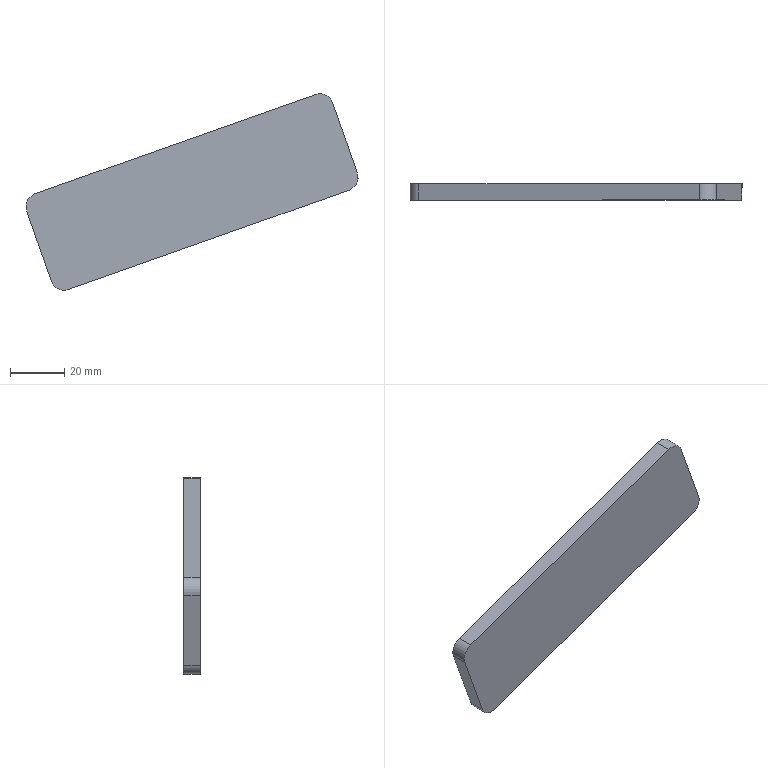Part | STEP file | WEAR-PLATE1_id190_x_t | 1 solid | 10 faces | box 122.87 x 6 x 72.641 mm | volume 26871 mm3 | plane 6 | cylinder 4 | commonest cylinder face diameters 10 x4
STEP:
#1=CARTESIAN_POINT('',(55.133,-66.,-32.227));
#2=VERTEX_POINT('',#1);
#3=CARTESIAN_POINT('',(64.313,-66.,-58.15));
#4=VERTEX_POINT('',#3);
#5=CARTESIAN_POINT('',(55.133,-66.,-32.227));
#6=DIRECTION('',(0.3338,0.,-0.9426));
#7=VECTOR('',#6,1.);
#8=LINE('',#5,#7);
#9=EDGE_CURVE('',#2,#4,#8,.T.);
#10=ORIENTED_EDGE('',*,*,#9,.F.);
#11=CARTESIAN_POINT('',(48.751,-66.,-29.183));
#12=VERTEX_POINT('',#11);
#13=CARTESIAN_POINT('',(50.42,-66.,-33.896));
#14=DIRECTION('',(0.,1.,0.));
#15=DIRECTION('',(0.,0.,1.));
#16=AXIS2_PLACEMENT_3D('',#13,#14,#15);
#17=CIRCLE('',#16,5.);
#18=EDGE_CURVE('',#12,#2,#17,.T.);
#19=ORIENTED_EDGE('',*,*,#18,.F.);
#20=CARTESIAN_POINT('',(-54.939,-66.,-65.902));
#21=VERTEX_POINT('',#20);
#22=CARTESIAN_POINT('',(-54.939,-66.,-65.902));
#23=DIRECTION('',(0.9426,0.,0.3338));
#24=VECTOR('',#23,1.);
#25=LINE('',#22,#24);
#26=EDGE_CURVE('',#21,#12,#25,.T.);
#27=ORIENTED_EDGE('',*,*,#26,.F.);
#28=CARTESIAN_POINT('',(-57.984,-66.,-72.284));
#29=VERTEX_POINT('',#28);
#30=CARTESIAN_POINT('',(-53.27,-66.,-70.615));
#31=DIRECTION('',(0.,1.,0.));
#32=DIRECTION('',(0.,0.,1.));
#33=AXIS2_PLACEMENT_3D('',#30,#31,#32);
#34=CIRCLE('',#33,5.);
#35=EDGE_CURVE('',#29,#21,#34,.T.);
#36=ORIENTED_EDGE('',*,*,#35,.F.);
#37=CARTESIAN_POINT('',(-48.804,-66.,-98.207));
#38=VERTEX_POINT('',#37);
#39=CARTESIAN_POINT('',(-48.804,-66.,-98.207));
#40=DIRECTION('',(-0.3338,0.,0.9426));
#41=VECTOR('',#40,1.);
#42=LINE('',#39,#41);
#43=EDGE_CURVE('',#38,#29,#42,.T.);
#44=ORIENTED_EDGE('',*,*,#43,.F.);
#45=CARTESIAN_POINT('',(-42.422,-66.,-101.251));
#46=VERTEX_POINT('',#45);
#47=CARTESIAN_POINT('',(-44.091,-66.,-96.538));
#48=DIRECTION('',(0.,1.,0.));
#49=DIRECTION('',(0.,0.,1.));
#50=AXIS2_PLACEMENT_3D('',#47,#48,#49);
#51=CIRCLE('',#50,5.);
#52=EDGE_CURVE('',#46,#38,#51,.T.);
#53=ORIENTED_EDGE('',*,*,#52,.F.);
#54=CARTESIAN_POINT('',(61.269,-66.,-64.532));
#55=VERTEX_POINT('',#54);
#56=CARTESIAN_POINT('',(61.269,-66.,-64.532));
#57=DIRECTION('',(-0.9426,0.,-0.3338));
#58=VECTOR('',#57,1.);
#59=LINE('',#56,#58);
#60=EDGE_CURVE('',#55,#46,#59,.T.);
#61=ORIENTED_EDGE('',*,*,#60,.F.);
#62=CARTESIAN_POINT('',(59.6,-66.,-59.819));
#63=DIRECTION('',(0.,1.,0.));
#64=DIRECTION('',(0.,0.,1.));
#65=AXIS2_PLACEMENT_3D('',#62,#63,#64);
#66=CIRCLE('',#65,5.);
#67=EDGE_CURVE('',#4,#55,#66,.T.);
#68=ORIENTED_EDGE('',*,*,#67,.F.);
#69=EDGE_LOOP('',(#10,#19,#27,#36,#44,#53,#61,#68));
#70=FACE_OUTER_BOUND('',#69,.T.);
#71=CARTESIAN_POINT('',(-200.,-66.,-275.));
#72=DIRECTION('',(0.,1.,0.));
#73=DIRECTION('',(0.,0.,1.));
#74=AXIS2_PLACEMENT_3D('',#71,#72,#73);
#75=PLANE('',#74);
#76=ADVANCED_FACE('',(#70),#75,.F.);
#77=CARTESIAN_POINT('',(61.269,-60.,-64.532));
#78=VERTEX_POINT('',#77);
#79=CARTESIAN_POINT('',(61.269,-66.,-64.532));
#80=DIRECTION('',(0.,1.,0.));
#81=VECTOR('',#80,1.);
#82=LINE('',#79,#81);
#83=EDGE_CURVE('',#55,#78,#82,.T.);
#84=ORIENTED_EDGE('',*,*,#83,.F.);
#85=ORIENTED_EDGE('',*,*,#60,.T.);
#86=CARTESIAN_POINT('',(-42.422,-60.,-101.251));
#87=VERTEX_POINT('',#86);
#88=CARTESIAN_POINT('',(-42.422,-66.,-101.251));
#89=DIRECTION('',(0.,-1.,0.));
#90=VECTOR('',#89,1.);
#91=LINE('',#88,#90);
#92=EDGE_CURVE('',#87,#46,#91,.T.);
#93=ORIENTED_EDGE('',*,*,#92,.F.);
#94=CARTESIAN_POINT('',(-42.422,-60.,-101.251));
#95=DIRECTION('',(0.9426,0.,0.3338));
#96=VECTOR('',#95,1.);
#97=LINE('',#94,#96);
#98=EDGE_CURVE('',#87,#78,#97,.T.);
#99=ORIENTED_EDGE('',*,*,#98,.T.);
#100=EDGE_LOOP('',(#84,#85,#93,#99));
#101=FACE_OUTER_BOUND('',#100,.T.);
#102=CARTESIAN_POINT('',(61.269,-66.,-64.532));
#103=DIRECTION('',(0.3338,0.,-0.9426));
#104=DIRECTION('',(-0.9426,0.,-0.3338));
#105=AXIS2_PLACEMENT_3D('',#102,#103,#104);
#106=PLANE('',#105);
#107=ADVANCED_FACE('',(#101),#106,.T.);
#108=CARTESIAN_POINT('',(64.313,-60.,-58.15));
#109=VERTEX_POINT('',#108);
#110=CARTESIAN_POINT('',(64.313,-66.,-58.15));
#111=DIRECTION('',(0.,1.,0.));
#112=VECTOR('',#111,1.);
#113=LINE('',#110,#112);
#114=EDGE_CURVE('',#4,#109,#113,.T.);
#115=ORIENTED_EDGE('',*,*,#114,.F.);
#116=ORIENTED_EDGE('',*,*,#67,.T.);
#117=ORIENTED_EDGE('',*,*,#83,.T.);
#118=CARTESIAN_POINT('',(59.6,-60.,-59.819));
#119=DIRECTION('',(0.,-1.,0.));
#120=DIRECTION('',(0.,0.,1.));
#121=AXIS2_PLACEMENT_3D('',#118,#119,#120);
#122=CIRCLE('',#121,5.);
#123=EDGE_CURVE('',#78,#109,#122,.T.);
#124=ORIENTED_EDGE('',*,*,#123,.T.);
#125=EDGE_LOOP('',(#115,#116,#117,#124));
#126=FACE_OUTER_BOUND('',#125,.T.);
#127=CARTESIAN_POINT('',(59.6,-66.,-59.819));
#128=DIRECTION('',(0.,1.,0.));
#129=DIRECTION('',(0.,0.,1.));
#130=AXIS2_PLACEMENT_3D('',#127,#128,#129);
#131=CYLINDRICAL_SURFACE('',#130,5.);
#132=ADVANCED_FACE('',(#126),#131,.T.);
#133=CARTESIAN_POINT('',(55.133,-60.,-32.227));
#134=VERTEX_POINT('',#133);
#135=CARTESIAN_POINT('',(55.133,-66.,-32.227));
#136=DIRECTION('',(0.,1.,0.));
#137=VECTOR('',#136,1.);
#138=LINE('',#135,#137);
#139=EDGE_CURVE('',#2,#134,#138,.T.);
#140=ORIENTED_EDGE('',*,*,#139,.F.);
#141=ORIENTED_EDGE('',*,*,#9,.T.);
#142=ORIENTED_EDGE('',*,*,#114,.T.);
#143=CARTESIAN_POINT('',(64.313,-60.,-58.15));
#144=DIRECTION('',(-0.3338,0.,0.9426));
#145=VECTOR('',#144,1.);
#146=LINE('',#143,#145);
#147=EDGE_CURVE('',#109,#134,#146,.T.);
#148=ORIENTED_EDGE('',*,*,#147,.T.);
#149=EDGE_LOOP('',(#140,#141,#142,#148));
#150=FACE_OUTER_BOUND('',#149,.T.);
#151=CARTESIAN_POINT('',(55.133,-66.,-32.227));
#152=DIRECTION('',(0.9426,0.,0.3338));
#153=DIRECTION('',(0.3338,0.,-0.9426));
#154=AXIS2_PLACEMENT_3D('',#151,#152,#153);
#155=PLANE('',#154);
#156=ADVANCED_FACE('',(#150),#155,.T.);
#157=CARTESIAN_POINT('',(48.751,-60.,-29.183));
#158=VERTEX_POINT('',#157);
#159=CARTESIAN_POINT('',(48.751,-66.,-29.183));
#160=DIRECTION('',(0.,1.,0.));
#161=VECTOR('',#160,1.);
#162=LINE('',#159,#161);
#163=EDGE_CURVE('',#12,#158,#162,.T.);
#164=ORIENTED_EDGE('',*,*,#163,.F.);
#165=ORIENTED_EDGE('',*,*,#18,.T.);
#166=ORIENTED_EDGE('',*,*,#139,.T.);
#167=CARTESIAN_POINT('',(50.42,-60.,-33.896));
#168=DIRECTION('',(0.,-1.,0.));
#169=DIRECTION('',(0.,0.,1.));
#170=AXIS2_PLACEMENT_3D('',#167,#168,#169);
#171=CIRCLE('',#170,5.);
#172=EDGE_CURVE('',#134,#158,#171,.T.);
#173=ORIENTED_EDGE('',*,*,#172,.T.);
#174=EDGE_LOOP('',(#164,#165,#166,#173));
#175=FACE_OUTER_BOUND('',#174,.T.);
#176=CARTESIAN_POINT('',(50.42,-66.,-33.896));
#177=DIRECTION('',(0.,1.,0.));
#178=DIRECTION('',(0.,0.,1.));
#179=AXIS2_PLACEMENT_3D('',#176,#177,#178);
#180=CYLINDRICAL_SURFACE('',#179,5.);
#181=ADVANCED_FACE('',(#175),#180,.T.);
#182=CARTESIAN_POINT('',(-54.939,-60.,-65.902));
#183=VERTEX_POINT('',#182);
#184=CARTESIAN_POINT('',(-54.939,-66.,-65.902));
#185=DIRECTION('',(0.,1.,0.));
#186=VECTOR('',#185,1.);
#187=LINE('',#184,#186);
#188=EDGE_CURVE('',#21,#183,#187,.T.);
#189=ORIENTED_EDGE('',*,*,#188,.F.);
#190=ORIENTED_EDGE('',*,*,#26,.T.);
#191=ORIENTED_EDGE('',*,*,#163,.T.);
#192=CARTESIAN_POINT('',(48.751,-60.,-29.183));
#193=DIRECTION('',(-0.9426,0.,-0.3338));
#194=VECTOR('',#193,1.);
#195=LINE('',#192,#194);
#196=EDGE_CURVE('',#158,#183,#195,.T.);
#197=ORIENTED_EDGE('',*,*,#196,.T.);
#198=EDGE_LOOP('',(#189,#190,#191,#197));
#199=FACE_OUTER_BOUND('',#198,.T.);
#200=CARTESIAN_POINT('',(-54.939,-66.,-65.902));
#201=DIRECTION('',(-0.3338,0.,0.9426));
#202=DIRECTION('',(0.9426,0.,0.3338));
#203=AXIS2_PLACEMENT_3D('',#200,#201,#202);
#204=PLANE('',#203);
#205=ADVANCED_FACE('',(#199),#204,.T.);
#206=CARTESIAN_POINT('',(-57.984,-60.,-72.284));
#207=VERTEX_POINT('',#206);
#208=CARTESIAN_POINT('',(-57.984,-66.,-72.284));
#209=DIRECTION('',(0.,1.,0.));
#210=VECTOR('',#209,1.);
#211=LINE('',#208,#210);
#212=EDGE_CURVE('',#29,#207,#211,.T.);
#213=ORIENTED_EDGE('',*,*,#212,.F.);
#214=ORIENTED_EDGE('',*,*,#35,.T.);
#215=ORIENTED_EDGE('',*,*,#188,.T.);
#216=CARTESIAN_POINT('',(-53.27,-60.,-70.615));
#217=DIRECTION('',(0.,-1.,0.));
#218=DIRECTION('',(0.,0.,1.));
#219=AXIS2_PLACEMENT_3D('',#216,#217,#218);
#220=CIRCLE('',#219,5.);
#221=EDGE_CURVE('',#183,#207,#220,.T.);
#222=ORIENTED_EDGE('',*,*,#221,.T.);
#223=EDGE_LOOP('',(#213,#214,#215,#222));
#224=FACE_OUTER_BOUND('',#223,.T.);
#225=CARTESIAN_POINT('',(-53.27,-66.,-70.615));
#226=DIRECTION('',(0.,1.,0.));
#227=DIRECTION('',(0.,0.,1.));
#228=AXIS2_PLACEMENT_3D('',#225,#226,#227);
#229=CYLINDRICAL_SURFACE('',#228,5.);
#230=ADVANCED_FACE('',(#224),#229,.T.);
#231=CARTESIAN_POINT('',(-48.804,-60.,-98.207));
#232=VERTEX_POINT('',#231);
#233=CARTESIAN_POINT('',(-48.804,-66.,-98.207));
#234=DIRECTION('',(0.,1.,0.));
#235=VECTOR('',#234,1.);
#236=LINE('',#233,#235);
#237=EDGE_CURVE('',#38,#232,#236,.T.);
#238=ORIENTED_EDGE('',*,*,#237,.F.);
#239=ORIENTED_EDGE('',*,*,#43,.T.);
#240=ORIENTED_EDGE('',*,*,#212,.T.);
#241=CARTESIAN_POINT('',(-57.984,-60.,-72.284));
#242=DIRECTION('',(0.3338,0.,-0.9426));
#243=VECTOR('',#242,1.);
#244=LINE('',#241,#243);
#245=EDGE_CURVE('',#207,#232,#244,.T.);
#246=ORIENTED_EDGE('',*,*,#245,.T.);
#247=EDGE_LOOP('',(#238,#239,#240,#246));
#248=FACE_OUTER_BOUND('',#247,.T.);
#249=CARTESIAN_POINT('',(-48.804,-66.,-98.207));
#250=DIRECTION('',(-0.9426,0.,-0.3338));
#251=DIRECTION('',(-0.3338,0.,0.9426));
#252=AXIS2_PLACEMENT_3D('',#249,#250,#251);
#253=PLANE('',#252);
#254=ADVANCED_FACE('',(#248),#253,.T.);
#255=ORIENTED_EDGE('',*,*,#92,.T.);
#256=ORIENTED_EDGE('',*,*,#52,.T.);
#257=ORIENTED_EDGE('',*,*,#237,.T.);
#258=CARTESIAN_POINT('',(-44.091,-60.,-96.538));
#259=DIRECTION('',(0.,-1.,0.));
#260=DIRECTION('',(0.,0.,1.));
#261=AXIS2_PLACEMENT_3D('',#258,#259,#260);
#262=CIRCLE('',#261,5.);
#263=EDGE_CURVE('',#232,#87,#262,.T.);
#264=ORIENTED_EDGE('',*,*,#263,.T.);
#265=EDGE_LOOP('',(#255,#256,#257,#264));
#266=FACE_OUTER_BOUND('',#265,.T.);
#267=CARTESIAN_POINT('',(-44.091,-66.,-96.538));
#268=DIRECTION('',(0.,1.,0.));
#269=DIRECTION('',(0.,0.,1.));
#270=AXIS2_PLACEMENT_3D('',#267,#268,#269);
#271=CYLINDRICAL_SURFACE('',#270,5.);
#272=ADVANCED_FACE('',(#266),#271,.T.);
#273=ORIENTED_EDGE('',*,*,#245,.F.);
#274=ORIENTED_EDGE('',*,*,#221,.F.);
#275=ORIENTED_EDGE('',*,*,#196,.F.);
#276=ORIENTED_EDGE('',*,*,#172,.F.);
#277=ORIENTED_EDGE('',*,*,#147,.F.);
#278=ORIENTED_EDGE('',*,*,#123,.F.);
#279=ORIENTED_EDGE('',*,*,#98,.F.);
#280=ORIENTED_EDGE('',*,*,#263,.F.);
#281=EDGE_LOOP('',(#273,#274,#275,#276,#277,#278,#279,#280));
#282=FACE_OUTER_BOUND('',#281,.T.);
#283=CARTESIAN_POINT('',(-80.,-60.,-43.));
#284=DIRECTION('',(0.,-1.,0.));
#285=DIRECTION('',(0.,0.,-1.));
#286=AXIS2_PLACEMENT_3D('',#283,#284,#285);
#287=PLANE('',#286);
#288=ADVANCED_FACE('',(#282),#287,.F.);
#289=CLOSED_SHELL('',(#76,#107,#132,#156,#181,#205,#230,#254,#272,#288));
#290=MANIFOLD_SOLID_BREP('',#289);
#291=(LENGTH_UNIT()NAMED_UNIT(*)SI_UNIT(.MILLI.,.METRE.));
#292=UNCERTAINTY_MEASURE_WITH_UNIT(LENGTH_MEASURE(0.00002),#291,'','');
#293=(NAMED_UNIT(*)PLANE_ANGLE_UNIT()SI_UNIT($,.RADIAN.));
#294=PLANE_ANGLE_MEASURE_WITH_UNIT(PLANE_ANGLE_MEASURE(0.01745),#293);
#295=DIMENSIONAL_EXPONENTS(0.,0.,0.,0.,0.,0.,0.);
#296=(CONVERSION_BASED_UNIT('DEGREE',#294)NAMED_UNIT(#295)PLANE_ANGLE_UNIT());
#297=(NAMED_UNIT(*)SI_UNIT($,.STERADIAN.)SOLID_ANGLE_UNIT());
#298=(GEOMETRIC_REPRESENTATION_CONTEXT(3)GLOBAL_UNCERTAINTY_ASSIGNED_CONTEXT((#292))GLOBAL_UNIT_ASSIGNED_CONTEXT((#291,#296,#297))REPRESENTATION_CONTEXT('',''));
#299=ADVANCED_BREP_SHAPE_REPRESENTATION('',(#290),#298);